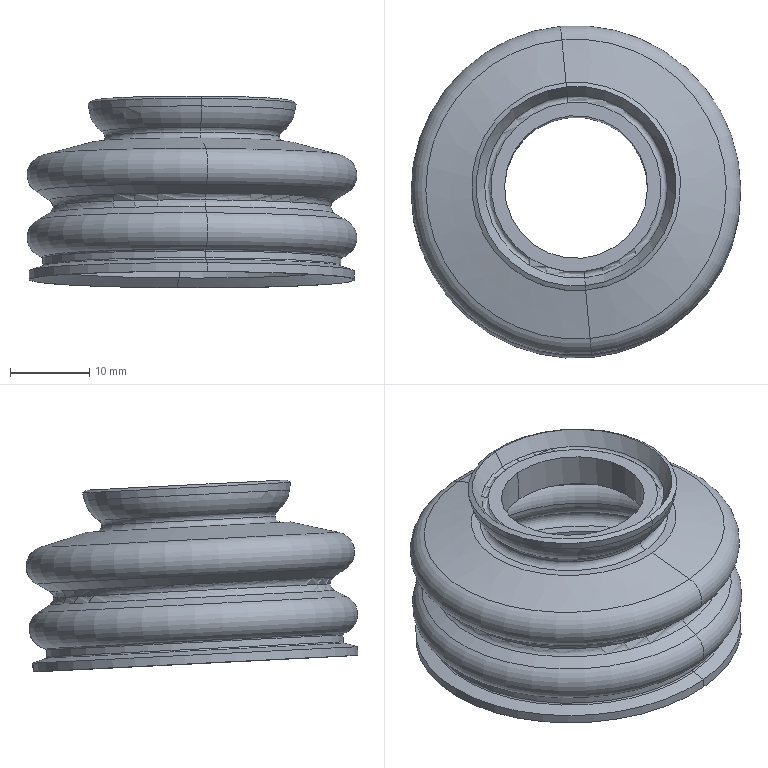Part | SolidWorks | features BaseBody 1 | 1 solid | 62 faces | box 41.506 x 41.869 x 24.152 mm | volume 5595 mm3 | torus 28 | cone 22 | cylinder 8 | plane 4 | commonest cylinder face diameters 18 x2 34 x2 37.5 x2 41 x2